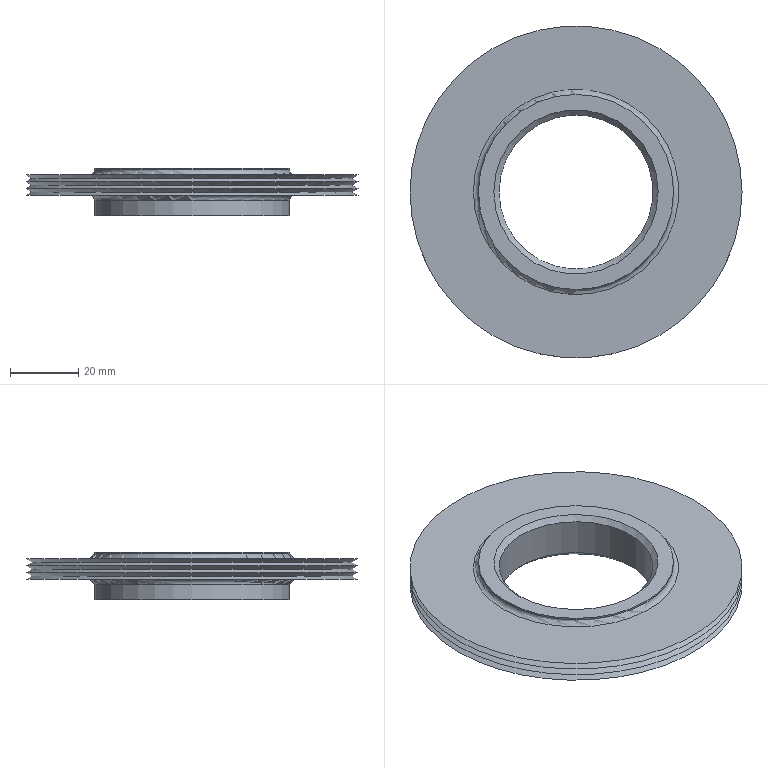Part | NX | features DATUM_CSYS 2, SKETCH 1, SWP104 1 | 1 solid | 17 faces | box 97 x 97 x 14 mm | volume 40772 mm3 | cone 8 | plane 4 | cylinder 3 | torus 2 | commonest cylinder face diameters 57 x2 45 x1
STEP:
#1=CARTESIAN_POINT('',(-48.5,0.,6.));
#2=VERTEX_POINT('',#1);
#3=CARTESIAN_POINT('',(0.,0.,6.));
#4=DIRECTION('',(0.,0.,-1.));
#5=DIRECTION('',(-1.,0.,0.));
#6=AXIS2_PLACEMENT_3D('',#3,#4,#5);
#7=CIRCLE('',#6,48.5);
#8=EDGE_CURVE('',#2,#2,#7,.T.);
#9=ORIENTED_EDGE('',*,*,#8,.F.);
#10=EDGE_LOOP('',(#9));
#11=FACE_BOUND('',#10,.T.);
#12=CARTESIAN_POINT('',(-46.768,0.,7.));
#13=VERTEX_POINT('',#12);
#14=CARTESIAN_POINT('',(0.,0.,7.));
#15=DIRECTION('',(0.,0.,-1.));
#16=DIRECTION('',(-1.,0.,0.));
#17=AXIS2_PLACEMENT_3D('',#14,#15,#16);
#18=CIRCLE('',#17,46.768);
#19=EDGE_CURVE('',#13,#13,#18,.T.);
#20=ORIENTED_EDGE('',*,*,#19,.T.);
#21=EDGE_LOOP('',(#20));
#22=FACE_BOUND('',#21,.T.);
#23=CARTESIAN_POINT('',(0.,0.,7.));
#24=DIRECTION('',(0.,0.,-1.));
#25=DIRECTION('',(-1.,0.,0.));
#26=AXIS2_PLACEMENT_3D('',#23,#24,#25);
#27=CONICAL_SURFACE('',#26,46.768,1.047);
#28=ADVANCED_FACE('',(#11,#22),#27,.T.);
#29=CARTESIAN_POINT('',(-30.,0.,6.));
#30=VERTEX_POINT('',#29);
#31=CARTESIAN_POINT('',(0.,0.,6.));
#32=DIRECTION('',(0.,0.,-1.));
#33=DIRECTION('',(-1.,0.,0.));
#34=AXIS2_PLACEMENT_3D('',#31,#32,#33);
#35=CIRCLE('',#34,30.);
#36=EDGE_CURVE('',#30,#30,#35,.T.);
#37=ORIENTED_EDGE('',*,*,#36,.F.);
#38=EDGE_LOOP('',(#37));
#39=FACE_BOUND('',#38,.T.);
#40=ORIENTED_EDGE('',*,*,#8,.T.);
#41=EDGE_LOOP('',(#40));
#42=FACE_BOUND('',#41,.T.);
#43=CARTESIAN_POINT('',(0.,-48.5,6.));
#44=DIRECTION('',(0.,0.,1.));
#45=DIRECTION('',(1.,0.,0.));
#46=AXIS2_PLACEMENT_3D('',#43,#44,#45);
#47=PLANE('',#46);
#48=ADVANCED_FACE('',(#39,#42),#47,.F.);
#49=CARTESIAN_POINT('',(-28.5,0.,4.5));
#50=VERTEX_POINT('',#49);
#51=CARTESIAN_POINT('',(0.,0.,4.5));
#52=DIRECTION('',(0.,0.,-1.));
#53=DIRECTION('',(-1.,0.,0.));
#54=AXIS2_PLACEMENT_3D('',#51,#52,#53);
#55=CIRCLE('',#54,28.5);
#56=EDGE_CURVE('',#50,#50,#55,.T.);
#57=ORIENTED_EDGE('',*,*,#56,.F.);
#58=EDGE_LOOP('',(#57));
#59=FACE_BOUND('',#58,.T.);
#60=ORIENTED_EDGE('',*,*,#36,.T.);
#61=EDGE_LOOP('',(#60));
#62=FACE_BOUND('',#61,.T.);
#63=CARTESIAN_POINT('',(0.,0.,4.5));
#64=DIRECTION('',(0.,0.,-1.));
#65=DIRECTION('',(-1.,0.,0.));
#66=AXIS2_PLACEMENT_3D('',#63,#64,#65);
#67=TOROIDAL_SURFACE('',#66,30.,1.5);
#68=ADVANCED_FACE('',(#59,#62),#67,.F.);
#69=CARTESIAN_POINT('',(-28.5,0.,0.));
#70=VERTEX_POINT('',#69);
#71=CARTESIAN_POINT('',(0.,0.,0.));
#72=DIRECTION('',(0.,0.,-1.));
#73=DIRECTION('',(-1.,0.,0.));
#74=AXIS2_PLACEMENT_3D('',#71,#72,#73);
#75=CIRCLE('',#74,28.5);
#76=EDGE_CURVE('',#70,#70,#75,.T.);
#77=ORIENTED_EDGE('',*,*,#76,.F.);
#78=EDGE_LOOP('',(#77));
#79=FACE_BOUND('',#78,.T.);
#80=ORIENTED_EDGE('',*,*,#56,.T.);
#81=EDGE_LOOP('',(#80));
#82=FACE_BOUND('',#81,.T.);
#83=CARTESIAN_POINT('',(0.,0.,0.));
#84=DIRECTION('',(0.,0.,-1.));
#85=DIRECTION('',(-1.,0.,0.));
#86=AXIS2_PLACEMENT_3D('',#83,#84,#85);
#87=CYLINDRICAL_SURFACE('',#86,28.5);
#88=ADVANCED_FACE('',(#79,#82),#87,.T.);
#89=CARTESIAN_POINT('',(-24.,0.,0.));
#90=VERTEX_POINT('',#89);
#91=CARTESIAN_POINT('',(0.,0.,0.));
#92=DIRECTION('',(0.,0.,-1.));
#93=DIRECTION('',(-1.,0.,0.));
#94=AXIS2_PLACEMENT_3D('',#91,#92,#93);
#95=CIRCLE('',#94,24.);
#96=EDGE_CURVE('',#90,#90,#95,.T.);
#97=ORIENTED_EDGE('',*,*,#96,.F.);
#98=EDGE_LOOP('',(#97));
#99=FACE_BOUND('',#98,.T.);
#100=ORIENTED_EDGE('',*,*,#76,.T.);
#101=EDGE_LOOP('',(#100));
#102=FACE_BOUND('',#101,.T.);
#103=CARTESIAN_POINT('',(0.,-28.5,0.));
#104=DIRECTION('',(0.,0.,1.));
#105=DIRECTION('',(1.,0.,0.));
#106=AXIS2_PLACEMENT_3D('',#103,#104,#105);
#107=PLANE('',#106);
#108=ADVANCED_FACE('',(#99,#102),#107,.F.);
#109=CARTESIAN_POINT('',(-22.5,0.,1.5));
#110=VERTEX_POINT('',#109);
#111=CARTESIAN_POINT('',(0.,0.,1.5));
#112=DIRECTION('',(0.,0.,-1.));
#113=DIRECTION('',(-1.,0.,0.));
#114=AXIS2_PLACEMENT_3D('',#111,#112,#113);
#115=CIRCLE('',#114,22.5);
#116=EDGE_CURVE('',#110,#110,#115,.T.);
#117=ORIENTED_EDGE('',*,*,#116,.F.);
#118=EDGE_LOOP('',(#117));
#119=FACE_BOUND('',#118,.T.);
#120=ORIENTED_EDGE('',*,*,#96,.T.);
#121=EDGE_LOOP('',(#120));
#122=FACE_BOUND('',#121,.T.);
#123=CARTESIAN_POINT('',(0.,0.,0.));
#124=DIRECTION('',(0.,0.,-1.));
#125=DIRECTION('',(-1.,0.,0.));
#126=AXIS2_PLACEMENT_3D('',#123,#124,#125);
#127=CONICAL_SURFACE('',#126,24.,0.7854);
#128=ADVANCED_FACE('',(#119,#122),#127,.F.);
#129=CARTESIAN_POINT('',(-22.5,0.,12.5));
#130=VERTEX_POINT('',#129);
#131=CARTESIAN_POINT('',(0.,0.,12.5));
#132=DIRECTION('',(0.,0.,-1.));
#133=DIRECTION('',(-1.,0.,0.));
#134=AXIS2_PLACEMENT_3D('',#131,#132,#133);
#135=CIRCLE('',#134,22.5);
#136=EDGE_CURVE('',#130,#130,#135,.T.);
#137=ORIENTED_EDGE('',*,*,#136,.F.);
#138=EDGE_LOOP('',(#137));
#139=FACE_BOUND('',#138,.T.);
#140=ORIENTED_EDGE('',*,*,#116,.T.);
#141=EDGE_LOOP('',(#140));
#142=FACE_BOUND('',#141,.T.);
#143=CARTESIAN_POINT('',(0.,0.,0.));
#144=DIRECTION('',(0.,0.,-1.));
#145=DIRECTION('',(-1.,0.,0.));
#146=AXIS2_PLACEMENT_3D('',#143,#144,#145);
#147=CYLINDRICAL_SURFACE('',#146,22.5);
#148=ADVANCED_FACE('',(#139,#142),#147,.F.);
#149=CARTESIAN_POINT('',(-24.,0.,14.));
#150=VERTEX_POINT('',#149);
#151=CARTESIAN_POINT('',(0.,0.,14.));
#152=DIRECTION('',(0.,0.,-1.));
#153=DIRECTION('',(-1.,0.,0.));
#154=AXIS2_PLACEMENT_3D('',#151,#152,#153);
#155=CIRCLE('',#154,24.);
#156=EDGE_CURVE('',#150,#150,#155,.T.);
#157=ORIENTED_EDGE('',*,*,#156,.F.);
#158=EDGE_LOOP('',(#157));
#159=FACE_BOUND('',#158,.T.);
#160=ORIENTED_EDGE('',*,*,#136,.T.);
#161=EDGE_LOOP('',(#160));
#162=FACE_BOUND('',#161,.T.);
#163=CARTESIAN_POINT('',(0.,0.,12.5));
#164=DIRECTION('',(0.,0.,1.));
#165=DIRECTION('',(1.,0.,0.));
#166=AXIS2_PLACEMENT_3D('',#163,#164,#165);
#167=CONICAL_SURFACE('',#166,22.5,0.7854);
#168=ADVANCED_FACE('',(#159,#162),#167,.F.);
#169=CARTESIAN_POINT('',(-28.5,0.,14.));
#170=VERTEX_POINT('',#169);
#171=CARTESIAN_POINT('',(0.,0.,14.));
#172=DIRECTION('',(0.,0.,-1.));
#173=DIRECTION('',(-1.,0.,0.));
#174=AXIS2_PLACEMENT_3D('',#171,#172,#173);
#175=CIRCLE('',#174,28.5);
#176=EDGE_CURVE('',#170,#170,#175,.T.);
#177=ORIENTED_EDGE('',*,*,#176,.F.);
#178=EDGE_LOOP('',(#177));
#179=FACE_BOUND('',#178,.T.);
#180=ORIENTED_EDGE('',*,*,#156,.T.);
#181=EDGE_LOOP('',(#180));
#182=FACE_BOUND('',#181,.T.);
#183=CARTESIAN_POINT('',(0.,-24.,14.));
#184=DIRECTION('',(0.,0.,-1.));
#185=DIRECTION('',(-1.,0.,0.));
#186=AXIS2_PLACEMENT_3D('',#183,#184,#185);
#187=PLANE('',#186);
#188=ADVANCED_FACE('',(#179,#182),#187,.F.);
#189=CARTESIAN_POINT('',(-28.5,0.,13.5));
#190=VERTEX_POINT('',#189);
#191=CARTESIAN_POINT('',(0.,0.,13.5));
#192=DIRECTION('',(0.,0.,-1.));
#193=DIRECTION('',(-1.,0.,0.));
#194=AXIS2_PLACEMENT_3D('',#191,#192,#193);
#195=CIRCLE('',#194,28.5);
#196=EDGE_CURVE('',#190,#190,#195,.T.);
#197=ORIENTED_EDGE('',*,*,#196,.F.);
#198=EDGE_LOOP('',(#197));
#199=FACE_BOUND('',#198,.T.);
#200=ORIENTED_EDGE('',*,*,#176,.T.);
#201=EDGE_LOOP('',(#200));
#202=FACE_BOUND('',#201,.T.);
#203=CARTESIAN_POINT('',(0.,0.,0.));
#204=DIRECTION('',(0.,0.,-1.));
#205=DIRECTION('',(-1.,0.,0.));
#206=AXIS2_PLACEMENT_3D('',#203,#204,#205);
#207=CYLINDRICAL_SURFACE('',#206,28.5);
#208=ADVANCED_FACE('',(#199,#202),#207,.T.);
#209=CARTESIAN_POINT('',(-30.,0.,12.));
#210=VERTEX_POINT('',#209);
#211=CARTESIAN_POINT('',(0.,0.,12.));
#212=DIRECTION('',(0.,0.,-1.));
#213=DIRECTION('',(-1.,0.,0.));
#214=AXIS2_PLACEMENT_3D('',#211,#212,#213);
#215=CIRCLE('',#214,30.);
#216=EDGE_CURVE('',#210,#210,#215,.T.);
#217=ORIENTED_EDGE('',*,*,#216,.F.);
#218=EDGE_LOOP('',(#217));
#219=FACE_BOUND('',#218,.T.);
#220=ORIENTED_EDGE('',*,*,#196,.T.);
#221=EDGE_LOOP('',(#220));
#222=FACE_BOUND('',#221,.T.);
#223=CARTESIAN_POINT('',(0.,0.,13.5));
#224=DIRECTION('',(0.,0.,-1.));
#225=DIRECTION('',(-1.,0.,0.));
#226=AXIS2_PLACEMENT_3D('',#223,#224,#225);
#227=TOROIDAL_SURFACE('',#226,30.,1.5);
#228=ADVANCED_FACE('',(#219,#222),#227,.F.);
#229=CARTESIAN_POINT('',(-48.5,0.,12.));
#230=VERTEX_POINT('',#229);
#231=CARTESIAN_POINT('',(0.,0.,12.));
#232=DIRECTION('',(0.,0.,-1.));
#233=DIRECTION('',(-1.,0.,0.));
#234=AXIS2_PLACEMENT_3D('',#231,#232,#233);
#235=CIRCLE('',#234,48.5);
#236=EDGE_CURVE('',#230,#230,#235,.T.);
#237=ORIENTED_EDGE('',*,*,#236,.F.);
#238=EDGE_LOOP('',(#237));
#239=FACE_BOUND('',#238,.T.);
#240=ORIENTED_EDGE('',*,*,#216,.T.);
#241=EDGE_LOOP('',(#240));
#242=FACE_BOUND('',#241,.T.);
#243=CARTESIAN_POINT('',(0.,-30.,12.));
#244=DIRECTION('',(0.,0.,-1.));
#245=DIRECTION('',(-1.,0.,0.));
#246=AXIS2_PLACEMENT_3D('',#243,#244,#245);
#247=PLANE('',#246);
#248=ADVANCED_FACE('',(#239,#242),#247,.F.);
#249=CARTESIAN_POINT('',(-46.768,0.,11.));
#250=VERTEX_POINT('',#249);
#251=CARTESIAN_POINT('',(0.,0.,11.));
#252=DIRECTION('',(0.,0.,-1.));
#253=DIRECTION('',(-1.,0.,0.));
#254=AXIS2_PLACEMENT_3D('',#251,#252,#253);
#255=CIRCLE('',#254,46.768);
#256=EDGE_CURVE('',#250,#250,#255,.T.);
#257=ORIENTED_EDGE('',*,*,#256,.F.);
#258=EDGE_LOOP('',(#257));
#259=FACE_BOUND('',#258,.T.);
#260=ORIENTED_EDGE('',*,*,#236,.T.);
#261=EDGE_LOOP('',(#260));
#262=FACE_BOUND('',#261,.T.);
#263=CARTESIAN_POINT('',(0.,0.,12.));
#264=DIRECTION('',(0.,0.,1.));
#265=DIRECTION('',(1.,0.,0.));
#266=AXIS2_PLACEMENT_3D('',#263,#264,#265);
#267=CONICAL_SURFACE('',#266,48.5,1.047);
#268=ADVANCED_FACE('',(#259,#262),#267,.T.);
#269=CARTESIAN_POINT('',(-48.5,0.,10.));
#270=VERTEX_POINT('',#269);
#271=CARTESIAN_POINT('',(0.,0.,10.));
#272=DIRECTION('',(0.,0.,-1.));
#273=DIRECTION('',(-1.,0.,0.));
#274=AXIS2_PLACEMENT_3D('',#271,#272,#273);
#275=CIRCLE('',#274,48.5);
#276=EDGE_CURVE('',#270,#270,#275,.T.);
#277=ORIENTED_EDGE('',*,*,#276,.F.);
#278=EDGE_LOOP('',(#277));
#279=FACE_BOUND('',#278,.T.);
#280=ORIENTED_EDGE('',*,*,#256,.T.);
#281=EDGE_LOOP('',(#280));
#282=FACE_BOUND('',#281,.T.);
#283=CARTESIAN_POINT('',(0.,0.,11.));
#284=DIRECTION('',(0.,0.,-1.));
#285=DIRECTION('',(-1.,0.,0.));
#286=AXIS2_PLACEMENT_3D('',#283,#284,#285);
#287=CONICAL_SURFACE('',#286,46.768,1.047);
#288=ADVANCED_FACE('',(#279,#282),#287,.T.);
#289=CARTESIAN_POINT('',(-46.768,0.,9.));
#290=VERTEX_POINT('',#289);
#291=CARTESIAN_POINT('',(0.,0.,9.));
#292=DIRECTION('',(0.,0.,-1.));
#293=DIRECTION('',(-1.,0.,0.));
#294=AXIS2_PLACEMENT_3D('',#291,#292,#293);
#295=CIRCLE('',#294,46.768);
#296=EDGE_CURVE('',#290,#290,#295,.T.);
#297=ORIENTED_EDGE('',*,*,#296,.F.);
#298=EDGE_LOOP('',(#297));
#299=FACE_BOUND('',#298,.T.);
#300=ORIENTED_EDGE('',*,*,#276,.T.);
#301=EDGE_LOOP('',(#300));
#302=FACE_BOUND('',#301,.T.);
#303=CARTESIAN_POINT('',(0.,0.,10.));
#304=DIRECTION('',(0.,0.,1.));
#305=DIRECTION('',(1.,0.,0.));
#306=AXIS2_PLACEMENT_3D('',#303,#304,#305);
#307=CONICAL_SURFACE('',#306,48.5,1.047);
#308=ADVANCED_FACE('',(#299,#302),#307,.T.);
#309=CARTESIAN_POINT('',(-48.5,0.,8.));
#310=VERTEX_POINT('',#309);
#311=CARTESIAN_POINT('',(0.,0.,8.));
#312=DIRECTION('',(0.,0.,-1.));
#313=DIRECTION('',(-1.,0.,0.));
#314=AXIS2_PLACEMENT_3D('',#311,#312,#313);
#315=CIRCLE('',#314,48.5);
#316=EDGE_CURVE('',#310,#310,#315,.T.);
#317=ORIENTED_EDGE('',*,*,#316,.F.);
#318=EDGE_LOOP('',(#317));
#319=FACE_BOUND('',#318,.T.);
#320=ORIENTED_EDGE('',*,*,#296,.T.);
#321=EDGE_LOOP('',(#320));
#322=FACE_BOUND('',#321,.T.);
#323=CARTESIAN_POINT('',(0.,0.,9.));
#324=DIRECTION('',(0.,0.,-1.));
#325=DIRECTION('',(-1.,0.,0.));
#326=AXIS2_PLACEMENT_3D('',#323,#324,#325);
#327=CONICAL_SURFACE('',#326,46.768,1.047);
#328=ADVANCED_FACE('',(#319,#322),#327,.T.);
#329=ORIENTED_EDGE('',*,*,#19,.F.);
#330=EDGE_LOOP('',(#329));
#331=FACE_BOUND('',#330,.T.);
#332=ORIENTED_EDGE('',*,*,#316,.T.);
#333=EDGE_LOOP('',(#332));
#334=FACE_BOUND('',#333,.T.);
#335=CARTESIAN_POINT('',(0.,0.,8.));
#336=DIRECTION('',(0.,0.,1.));
#337=DIRECTION('',(1.,0.,0.));
#338=AXIS2_PLACEMENT_3D('',#335,#336,#337);
#339=CONICAL_SURFACE('',#338,48.5,1.047);
#340=ADVANCED_FACE('',(#331,#334),#339,.T.);
#341=CLOSED_SHELL('',(#28,#48,#68,#88,#108,#128,#148,#168,#188,#208,#228,#248,#268,#288,#308,#328,#340));
#342=MANIFOLD_SOLID_BREP('',#341);
#343=(LENGTH_UNIT()NAMED_UNIT(*)SI_UNIT(.MILLI.,.METRE.));
#344=UNCERTAINTY_MEASURE_WITH_UNIT(LENGTH_MEASURE(0.00001),#343,'','');
#345=(NAMED_UNIT(*)PLANE_ANGLE_UNIT()SI_UNIT($,.RADIAN.));
#346=(NAMED_UNIT(*)SI_UNIT($,.STERADIAN.)SOLID_ANGLE_UNIT());
#347=(GEOMETRIC_REPRESENTATION_CONTEXT(3)GLOBAL_UNCERTAINTY_ASSIGNED_CONTEXT((#344))GLOBAL_UNIT_ASSIGNED_CONTEXT((#343,#345,#346))REPRESENTATION_CONTEXT('',''));
#348=ADVANCED_BREP_SHAPE_REPRESENTATION('',(#342),#347);